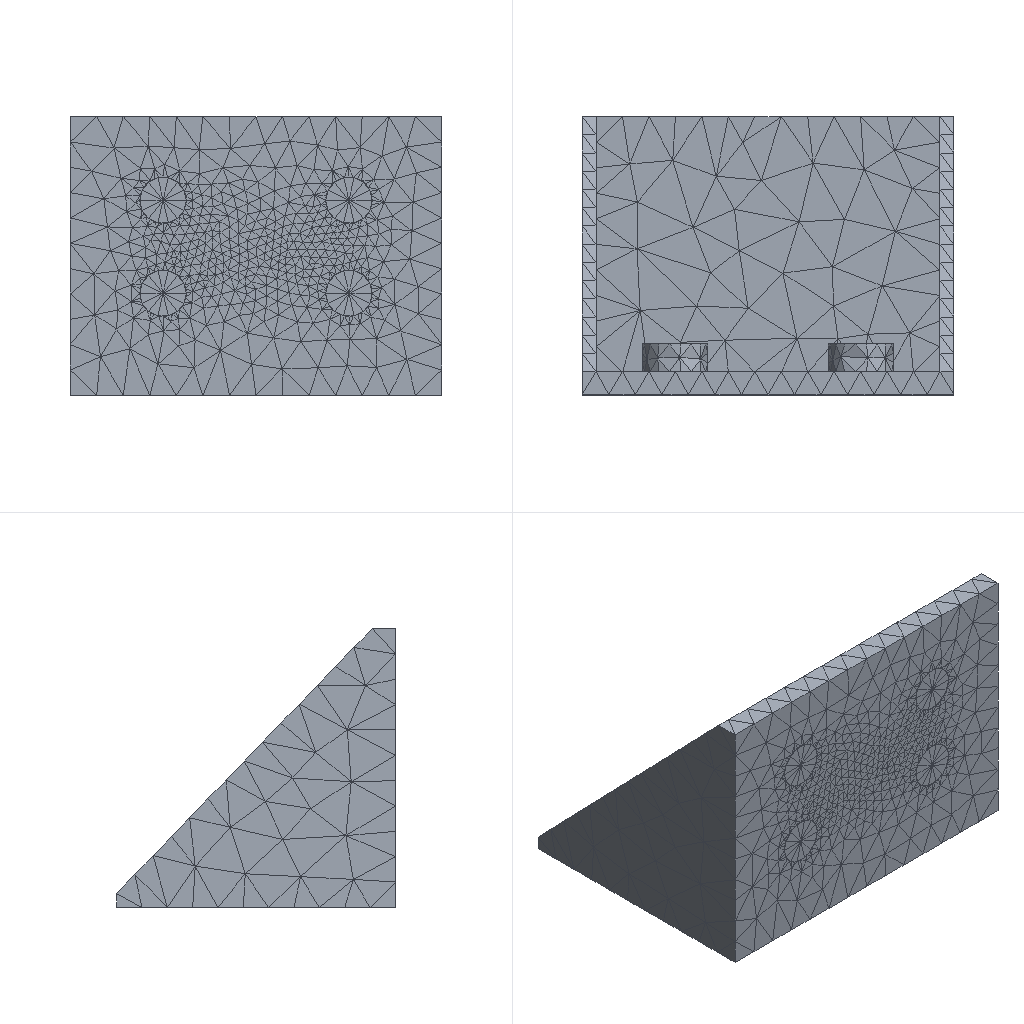Simulation study | ansys workbench
Set-up summary:
category,name,step,type,value,unit,region
solver,ansys_mapdl
solver,version,,,22.1
solver,version,,,22.1
solver,version,,,22.1
solver,version,,,22.1
units,MPA,,stated
analysis,deck1,,modal,modal
load_step,requested,,,2
analysis,nlgeom,,,False
mesh,nodes,,,0
mesh,elements,,,0
load,load commands in deck,,count,0
bc,support commands in deck,,count,0
analysis,deck2,,static,static
load_step,requested,,,1
analysis,nlgeom,,,False
mesh,nodes,,,16363
mesh,elements,,,11888
element_type,ANSYS 187 (type 1),,solid,7672
element_type,ANSYS 187 (type 2),,solid,280
element_type,ANSYS 187 (type 3),,solid,270
element_type,ANSYS 187 (type 4),,solid,268
element_type,ANSYS 187 (type 5),,solid,278
element_type,ANSYS 174 (type 6),,contact,1504
element_type,ANSYS 170 (type 7),,target,1504
element_type,ANSYS 154 (type 8),,surface,112
load,load commands in deck,,count,3
bc,support commands in deck,,count,1
named_set,_CM57_FIXEDSU,,component
named_set,_CM59_FIXEDSU,,component
named_set,_FIXEDSU,,component
material,1,,in results
material,2,,in results
material,3,,in results
material,4,,in results
material,5,,in results
material,1,,in results
material,2,,in results
material,4,,in results
material,5,,in results
material,1,,in results
material,3,,in results
material,1,,in results
material,2,,in results
material,3,,in results
material,4,,in results
material,5,,in results
check,setup vs results,,match,112 surface effect element(s) are not in the reader's mesh and were not compared
check,setup vs results,,match,112 surface effect element(s) are not in the reader's mesh and were not compared
Results summary:
result,analysis,,,modal
result,last_loadstep,,,1
result,primary field,,,displacement
result,analysis,,,static
result,last_loadstep,,,1
result,primary field,,,displacement
result,reaction total,1,FX,-8.231,N
result,reaction total,1,FY,-0.06635,N
result,reaction total,1,FZ,-21.938,N
result,mass,,,0.01759,"NMM: mm, ton, N, s, mV, mA, degC"
result,analysis,,,static
result,last_loadstep,,,1
result,primary field,,,displacement
result,reaction total,1,FX,8.231,N
result,reaction total,1,FY,0.06635,N
result,reaction total,1,FZ,-22.062,N
result,mass,,,0.03177,"NMM: mm, ton, N, s, mV, mA, degC"
result,analysis,,,static
result,last_loadstep,,,1
result,primary field,,,displacement
result,reaction total,1,FX,-0.0,N
result,reaction total,1,FY,0.0,N
result,reaction total,1,FZ,-44.0,N
result,mass,,,0.04936,"NMM: mm, ton, N, s, mV, mA, degC"